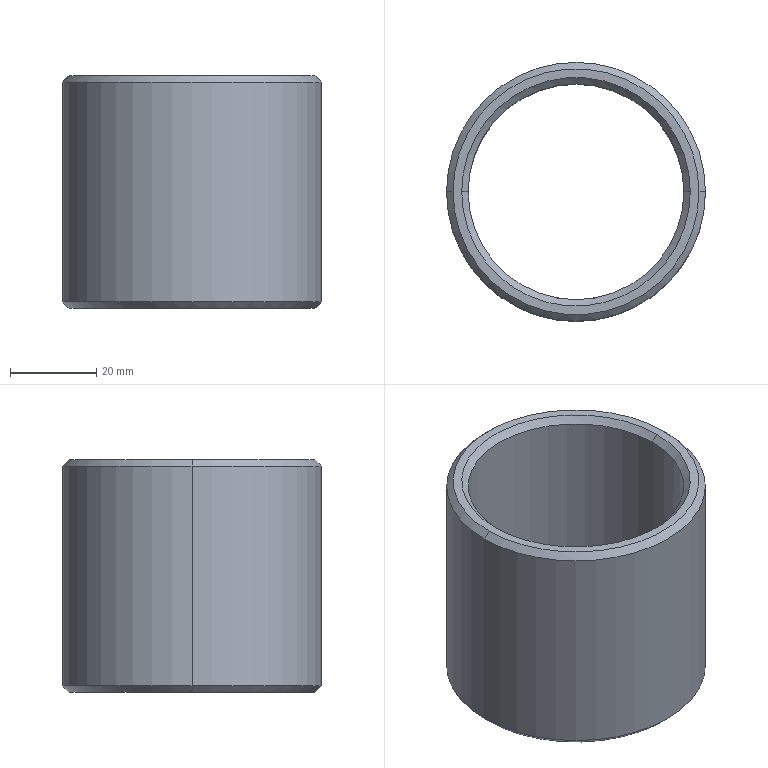Part | SolidWorks | features Chamfer 1, Extrusion 1, ICE 1, RevCut 1 | 1 solid | 18 faces | box 60 x 60 x 54 mm | volume 45325 mm3 | cone 9 | cylinder 5 | sphere 2 | plane 2 | commonest cylinder face diameters 50 x2 60 x2 6 x1
STEP:
#1=CARTESIAN_POINT('',(-25.,0.,25.5));
#2=VERTEX_POINT('',#1);
#3=CARTESIAN_POINT('',(25.,0.,25.5));
#4=VERTEX_POINT('',#3);
#5=CARTESIAN_POINT('',(0.,0.,25.5));
#6=DIRECTION('',(0.,0.,1.));
#7=DIRECTION('',(1.,0.,0.));
#8=AXIS2_PLACEMENT_3D('',#5,#6,#7);
#9=CIRCLE('',#8,25.);
#10=EDGE_CURVE('',#2,#4,#9,.T.);
#11=ORIENTED_EDGE('',*,*,#10,.F.);
#12=CARTESIAN_POINT('',(-26.5,0.,27.));
#13=VERTEX_POINT('',#12);
#14=CARTESIAN_POINT('',(-25.,0.,25.5));
#15=DIRECTION('',(-0.7071,0.,0.7071));
#16=VECTOR('',#15,1000.);
#17=LINE('',#14,#16);
#18=EDGE_CURVE('',#2,#13,#17,.T.);
#19=ORIENTED_EDGE('',*,*,#18,.T.);
#20=CARTESIAN_POINT('',(26.5,0.,27.));
#21=VERTEX_POINT('',#20);
#22=CARTESIAN_POINT('',(0.,0.,27.));
#23=DIRECTION('',(0.,0.,-1.));
#24=DIRECTION('',(1.,0.,0.));
#25=AXIS2_PLACEMENT_3D('',#22,#23,#24);
#26=CIRCLE('',#25,26.5);
#27=EDGE_CURVE('',#21,#13,#26,.T.);
#28=ORIENTED_EDGE('',*,*,#27,.F.);
#29=CARTESIAN_POINT('',(25.,0.,25.5));
#30=DIRECTION('',(0.7071,0.,0.7071));
#31=VECTOR('',#30,1000.);
#32=LINE('',#29,#31);
#33=EDGE_CURVE('',#4,#21,#32,.T.);
#34=ORIENTED_EDGE('',*,*,#33,.F.);
#35=EDGE_LOOP('',(#11,#19,#28,#34));
#36=FACE_OUTER_BOUND('',#35,.T.);
#37=CARTESIAN_POINT('',(0.,0.,25.5));
#38=DIRECTION('',(0.,0.,1.));
#39=DIRECTION('',(1.,0.,0.));
#40=AXIS2_PLACEMENT_3D('',#37,#38,#39);
#41=CONICAL_SURFACE('',#40,25.,0.7854);
#42=ADVANCED_FACE('',(#36),#41,.F.);
#43=CARTESIAN_POINT('',(28.5,0.,27.));
#44=VERTEX_POINT('',#43);
#45=CARTESIAN_POINT('',(-28.5,0.,27.));
#46=VERTEX_POINT('',#45);
#47=CARTESIAN_POINT('',(0.,0.,27.));
#48=DIRECTION('',(0.,0.,1.));
#49=DIRECTION('',(1.,0.,0.));
#50=AXIS2_PLACEMENT_3D('',#47,#48,#49);
#51=CIRCLE('',#50,28.5);
#52=EDGE_CURVE('',#44,#46,#51,.T.);
#53=ORIENTED_EDGE('',*,*,#52,.F.);
#54=CARTESIAN_POINT('',(30.,0.,25.5));
#55=VERTEX_POINT('',#54);
#56=CARTESIAN_POINT('',(28.5,0.,27.));
#57=DIRECTION('',(0.7071,0.,-0.7071));
#58=VECTOR('',#57,1000.);
#59=LINE('',#56,#58);
#60=EDGE_CURVE('',#44,#55,#59,.T.);
#61=ORIENTED_EDGE('',*,*,#60,.T.);
#62=CARTESIAN_POINT('',(-30.,0.,25.5));
#63=VERTEX_POINT('',#62);
#64=CARTESIAN_POINT('',(0.,0.,25.5));
#65=DIRECTION('',(0.,0.,-1.));
#66=DIRECTION('',(1.,0.,0.));
#67=AXIS2_PLACEMENT_3D('',#64,#65,#66);
#68=CIRCLE('',#67,30.);
#69=EDGE_CURVE('',#63,#55,#68,.T.);
#70=ORIENTED_EDGE('',*,*,#69,.F.);
#71=CARTESIAN_POINT('',(-28.5,0.,27.));
#72=DIRECTION('',(-0.7071,0.,-0.7071));
#73=VECTOR('',#72,1000.);
#74=LINE('',#71,#73);
#75=EDGE_CURVE('',#46,#63,#74,.T.);
#76=ORIENTED_EDGE('',*,*,#75,.F.);
#77=EDGE_LOOP('',(#53,#61,#70,#76));
#78=FACE_OUTER_BOUND('',#77,.T.);
#79=CARTESIAN_POINT('',(0.,0.,27.));
#80=DIRECTION('',(0.,0.,-1.));
#81=DIRECTION('',(-1.,0.,0.));
#82=AXIS2_PLACEMENT_3D('',#79,#80,#81);
#83=CONICAL_SURFACE('',#82,28.5,0.7854);
#84=ADVANCED_FACE('',(#78),#83,.T.);
#85=CARTESIAN_POINT('',(-28.5,0.,-27.));
#86=VERTEX_POINT('',#85);
#87=CARTESIAN_POINT('',(28.5,0.,-27.));
#88=VERTEX_POINT('',#87);
#89=CARTESIAN_POINT('',(0.,0.,-27.));
#90=DIRECTION('',(0.,0.,-1.));
#91=DIRECTION('',(1.,0.,0.));
#92=AXIS2_PLACEMENT_3D('',#89,#90,#91);
#93=CIRCLE('',#92,28.5);
#94=EDGE_CURVE('',#86,#88,#93,.T.);
#95=ORIENTED_EDGE('',*,*,#94,.F.);
#96=CARTESIAN_POINT('',(-30.,0.,-25.5));
#97=VERTEX_POINT('',#96);
#98=CARTESIAN_POINT('',(-30.,0.,-25.5));
#99=DIRECTION('',(-0.7071,0.,0.7071));
#100=VECTOR('',#99,1000.);
#101=LINE('',#98,#100);
#102=EDGE_CURVE('',#86,#97,#101,.T.);
#103=ORIENTED_EDGE('',*,*,#102,.T.);
#104=CARTESIAN_POINT('',(30.,0.,-25.5));
#105=VERTEX_POINT('',#104);
#106=CARTESIAN_POINT('',(0.,0.,-25.5));
#107=DIRECTION('',(0.,0.,1.));
#108=DIRECTION('',(1.,0.,0.));
#109=AXIS2_PLACEMENT_3D('',#106,#107,#108);
#110=CIRCLE('',#109,30.);
#111=EDGE_CURVE('',#105,#97,#110,.T.);
#112=ORIENTED_EDGE('',*,*,#111,.F.);
#113=CARTESIAN_POINT('',(30.,0.,-25.5));
#114=DIRECTION('',(0.7071,0.,0.7071));
#115=VECTOR('',#114,1000.);
#116=LINE('',#113,#115);
#117=EDGE_CURVE('',#88,#105,#116,.T.);
#118=ORIENTED_EDGE('',*,*,#117,.F.);
#119=EDGE_LOOP('',(#95,#103,#112,#118));
#120=FACE_OUTER_BOUND('',#119,.T.);
#121=CARTESIAN_POINT('',(0.,0.,-25.5));
#122=DIRECTION('',(0.,0.,1.));
#123=DIRECTION('',(1.,0.,0.));
#124=AXIS2_PLACEMENT_3D('',#121,#122,#123);
#125=CONICAL_SURFACE('',#124,30.,0.7854);
#126=ADVANCED_FACE('',(#120),#125,.T.);
#127=CARTESIAN_POINT('',(25.,0.,-25.5));
#128=VERTEX_POINT('',#127);
#129=CARTESIAN_POINT('',(2.983,-24.821,-25.5));
#130=VERTEX_POINT('',#129);
#131=CARTESIAN_POINT('',(0.,0.,-25.5));
#132=DIRECTION('',(0.,0.,-1.));
#133=DIRECTION('',(1.,0.,0.));
#134=AXIS2_PLACEMENT_3D('',#131,#132,#133);
#135=CIRCLE('',#134,25.);
#136=EDGE_CURVE('',#128,#130,#135,.T.);
#137=ORIENTED_EDGE('',*,*,#136,.F.);
#138=CARTESIAN_POINT('',(26.5,0.,-27.));
#139=VERTEX_POINT('',#138);
#140=CARTESIAN_POINT('',(26.5,0.,-27.));
#141=DIRECTION('',(0.7071,0.,-0.7071));
#142=VECTOR('',#141,1000.);
#143=LINE('',#140,#142);
#144=EDGE_CURVE('',#128,#139,#143,.T.);
#145=ORIENTED_EDGE('',*,*,#144,.T.);
#146=CARTESIAN_POINT('',(2.323,-26.398,-27.));
#147=VERTEX_POINT('',#146);
#148=CARTESIAN_POINT('',(0.,0.,-27.));
#149=DIRECTION('',(0.,0.,1.));
#150=DIRECTION('',(1.,0.,0.));
#151=AXIS2_PLACEMENT_3D('',#148,#149,#150);
#152=CIRCLE('',#151,26.5);
#153=EDGE_CURVE('',#147,#139,#152,.T.);
#154=ORIENTED_EDGE('',*,*,#153,.F.);
#155=CARTESIAN_POINT('',(2.323,-26.398,-27.));
#156=CARTESIAN_POINT('',(2.522,-26.155,-26.776));
#157=CARTESIAN_POINT('',(2.669,-25.899,-26.536));
#158=CARTESIAN_POINT('',(2.885,-25.37,-26.033));
#159=CARTESIAN_POINT('',(2.953,-25.095,-25.768));
#160=CARTESIAN_POINT('',(2.983,-24.821,-25.5));
#161=B_SPLINE_CURVE_WITH_KNOTS('',3,(#155,#156,#157,#158,#159,#160),.UNSPECIFIED.,.F.,.F.,(4,2,4),(0.000000339,0.00114,0.00228),.UNSPECIFIED.);
#162=EDGE_CURVE('',#147,#130,#161,.T.);
#163=ORIENTED_EDGE('',*,*,#162,.T.);
#164=EDGE_LOOP('',(#137,#145,#154,#163));
#165=FACE_OUTER_BOUND('',#164,.T.);
#166=CARTESIAN_POINT('',(0.,0.,-27.));
#167=DIRECTION('',(0.,0.,-1.));
#168=DIRECTION('',(-1.,0.,0.));
#169=AXIS2_PLACEMENT_3D('',#166,#167,#168);
#170=CONICAL_SURFACE('',#169,26.5,0.7854);
#171=ADVANCED_FACE('',(#165),#170,.F.);
#172=ORIENTED_EDGE('',*,*,#144,.F.);
#173=CARTESIAN_POINT('',(-25.,0.,-25.5));
#174=VERTEX_POINT('',#173);
#175=CARTESIAN_POINT('',(0.,0.,-25.5));
#176=DIRECTION('',(0.,0.,-1.));
#177=DIRECTION('',(1.,0.,0.));
#178=AXIS2_PLACEMENT_3D('',#175,#176,#177);
#179=CIRCLE('',#178,25.);
#180=EDGE_CURVE('',#174,#128,#179,.T.);
#181=ORIENTED_EDGE('',*,*,#180,.F.);
#182=CARTESIAN_POINT('',(-26.5,0.,-27.));
#183=VERTEX_POINT('',#182);
#184=CARTESIAN_POINT('',(-26.5,0.,-27.));
#185=DIRECTION('',(-0.7071,0.,-0.7071));
#186=VECTOR('',#185,1000.);
#187=LINE('',#184,#186);
#188=EDGE_CURVE('',#174,#183,#187,.T.);
#189=ORIENTED_EDGE('',*,*,#188,.T.);
#190=CARTESIAN_POINT('',(0.,0.,-27.));
#191=DIRECTION('',(0.,0.,1.));
#192=DIRECTION('',(1.,0.,0.));
#193=AXIS2_PLACEMENT_3D('',#190,#191,#192);
#194=CIRCLE('',#193,26.5);
#195=EDGE_CURVE('',#139,#183,#194,.T.);
#196=ORIENTED_EDGE('',*,*,#195,.F.);
#197=EDGE_LOOP('',(#172,#181,#189,#196));
#198=FACE_OUTER_BOUND('',#197,.T.);
#199=CARTESIAN_POINT('',(0.,0.,-27.));
#200=DIRECTION('',(0.,0.,-1.));
#201=DIRECTION('',(-1.,0.,0.));
#202=AXIS2_PLACEMENT_3D('',#199,#200,#201);
#203=CONICAL_SURFACE('',#202,26.5,0.7854);
#204=ADVANCED_FACE('',(#198),#203,.F.);
#205=ORIENTED_EDGE('',*,*,#10,.T.);
#206=CARTESIAN_POINT('',(25.,0.,27.));
#207=DIRECTION('',(0.,0.,-1.));
#208=VECTOR('',#207,1000.);
#209=LINE('',#206,#208);
#210=EDGE_CURVE('',#4,#128,#209,.T.);
#211=ORIENTED_EDGE('',*,*,#210,.T.);
#212=ORIENTED_EDGE('',*,*,#136,.T.);
#213=CARTESIAN_POINT('',(2.983,-24.821,19.5));
#214=VERTEX_POINT('',#213);
#215=CARTESIAN_POINT('',(2.983,-24.821,0.));
#216=DIRECTION('',(0.,0.,1.));
#217=VECTOR('',#216,1000.);
#218=LINE('',#215,#217);
#219=EDGE_CURVE('',#130,#214,#218,.T.);
#220=ORIENTED_EDGE('',*,*,#219,.T.);
#221=CARTESIAN_POINT('',(0.,-25.,22.458));
#222=VERTEX_POINT('',#221);
#223=CARTESIAN_POINT('',(0.,-25.,22.458));
#224=CARTESIAN_POINT('',(0.1961,-25.,22.458));
#225=CARTESIAN_POINT('',(0.3891,-24.998,22.439));
#226=CARTESIAN_POINT('',(0.7692,-24.989,22.365));
#227=CARTESIAN_POINT('',(0.9582,-24.982,22.308));
#228=CARTESIAN_POINT('',(1.318,-24.966,22.161));
#229=CARTESIAN_POINT('',(1.489,-24.956,22.071));
#230=CARTESIAN_POINT('',(1.814,-24.935,21.858));
#231=CARTESIAN_POINT('',(1.967,-24.923,21.734));
#232=CARTESIAN_POINT('',(2.243,-24.9,21.462));
#233=CARTESIAN_POINT('',(2.366,-24.888,21.313));
#234=CARTESIAN_POINT('',(2.585,-24.866,20.99));
#235=CARTESIAN_POINT('',(2.678,-24.856,20.818));
#236=CARTESIAN_POINT('',(2.828,-24.84,20.461));
#237=CARTESIAN_POINT('',(2.886,-24.833,20.274));
#238=CARTESIAN_POINT('',(2.963,-24.824,19.891));
#239=CARTESIAN_POINT('',(2.983,-24.821,19.696));
#240=CARTESIAN_POINT('',(2.983,-24.821,19.5));
#241=B_SPLINE_CURVE_WITH_KNOTS('',3,(#223,#224,#225,#226,#227,#228,#229,#230,#231,#232,#233,#234,#235,#236,#237,#238,#239,#240),.UNSPECIFIED.,.F.,.F.,(4,2,2,2,2,2,2,2,4),(0.01395,0.01453,0.01511,0.01569,0.01627,0.01685,0.01743,0.01801,0.01859),.UNSPECIFIED.);
#242=EDGE_CURVE('',#222,#214,#241,.T.);
#243=ORIENTED_EDGE('',*,*,#242,.F.);
#244=CARTESIAN_POINT('',(-2.983,-24.821,19.5));
#245=VERTEX_POINT('',#244);
#246=CARTESIAN_POINT('',(-2.983,-24.821,19.5));
#247=CARTESIAN_POINT('',(-2.983,-24.821,19.694));
#248=CARTESIAN_POINT('',(-2.964,-24.824,19.887));
#249=CARTESIAN_POINT('',(-2.887,-24.833,20.271));
#250=CARTESIAN_POINT('',(-2.829,-24.84,20.458));
#251=CARTESIAN_POINT('',(-2.68,-24.856,20.815));
#252=CARTESIAN_POINT('',(-2.587,-24.866,20.988));
#253=CARTESIAN_POINT('',(-2.368,-24.888,21.311));
#254=CARTESIAN_POINT('',(-2.244,-24.899,21.46));
#255=CARTESIAN_POINT('',(-1.969,-24.923,21.732));
#256=CARTESIAN_POINT('',(-1.815,-24.935,21.857));
#257=CARTESIAN_POINT('',(-1.491,-24.956,22.07));
#258=CARTESIAN_POINT('',(-1.32,-24.966,22.161));
#259=CARTESIAN_POINT('',(-0.9588,-24.982,22.308));
#260=CARTESIAN_POINT('',(-0.7702,-24.989,22.364));
#261=CARTESIAN_POINT('',(-0.3901,-24.998,22.439));
#262=CARTESIAN_POINT('',(-0.1962,-25.,22.458));
#263=CARTESIAN_POINT('',(0.,-25.,22.458));
#264=B_SPLINE_CURVE_WITH_KNOTS('',3,(#246,#247,#248,#249,#250,#251,#252,#253,#254,#255,#256,#257,#258,#259,#260,#261,#262,#263),.UNSPECIFIED.,.F.,.F.,(4,2,2,2,2,2,2,2,4),(0.009298,0.009879,0.01046,0.01104,0.01162,0.0122,0.01278,0.01337,0.01395),.UNSPECIFIED.);
#265=EDGE_CURVE('',#245,#222,#264,.T.);
#266=ORIENTED_EDGE('',*,*,#265,.F.);
#267=CARTESIAN_POINT('',(-2.983,-24.821,-25.5));
#268=VERTEX_POINT('',#267);
#269=CARTESIAN_POINT('',(-2.983,-24.821,0.));
#270=DIRECTION('',(0.,0.,-1.));
#271=VECTOR('',#270,1000.);
#272=LINE('',#269,#271);
#273=EDGE_CURVE('',#245,#268,#272,.T.);
#274=ORIENTED_EDGE('',*,*,#273,.T.);
#275=CARTESIAN_POINT('',(0.,0.,-25.5));
#276=DIRECTION('',(0.,0.,-1.));
#277=DIRECTION('',(1.,0.,0.));
#278=AXIS2_PLACEMENT_3D('',#275,#276,#277);
#279=CIRCLE('',#278,25.);
#280=EDGE_CURVE('',#268,#174,#279,.T.);
#281=ORIENTED_EDGE('',*,*,#280,.T.);
#282=CARTESIAN_POINT('',(-25.,0.,27.));
#283=DIRECTION('',(0.,0.,-1.));
#284=VECTOR('',#283,1000.);
#285=LINE('',#282,#284);
#286=EDGE_CURVE('',#2,#174,#285,.T.);
#287=ORIENTED_EDGE('',*,*,#286,.F.);
#288=EDGE_LOOP('',(#205,#211,#212,#220,#243,#266,#274,#281,#287));
#289=FACE_OUTER_BOUND('',#288,.T.);
#290=CARTESIAN_POINT('',(0.,0.,27.));
#291=DIRECTION('',(0.,0.,-1.));
#292=DIRECTION('',(-1.,0.,0.));
#293=AXIS2_PLACEMENT_3D('',#290,#291,#292);
#294=CYLINDRICAL_SURFACE('',#293,25.);
#295=ADVANCED_FACE('',(#289),#294,.F.);
#296=ORIENTED_EDGE('',*,*,#69,.T.);
#297=CARTESIAN_POINT('',(30.,0.,27.));
#298=DIRECTION('',(0.,0.,-1.));
#299=VECTOR('',#298,1000.);
#300=LINE('',#297,#299);
#301=EDGE_CURVE('',#55,#105,#300,.T.);
#302=ORIENTED_EDGE('',*,*,#301,.T.);
#303=ORIENTED_EDGE('',*,*,#111,.T.);
#304=CARTESIAN_POINT('',(-30.,0.,27.));
#305=DIRECTION('',(0.,0.,-1.));
#306=VECTOR('',#305,1000.);
#307=LINE('',#304,#306);
#308=EDGE_CURVE('',#63,#97,#307,.T.);
#309=ORIENTED_EDGE('',*,*,#308,.F.);
#310=EDGE_LOOP('',(#296,#302,#303,#309));
#311=FACE_OUTER_BOUND('',#310,.T.);
#312=CARTESIAN_POINT('',(0.,0.,27.));
#313=DIRECTION('',(0.,0.,-1.));
#314=DIRECTION('',(-1.,0.,0.));
#315=AXIS2_PLACEMENT_3D('',#312,#313,#314);
#316=CYLINDRICAL_SURFACE('',#315,30.);
#317=ADVANCED_FACE('',(#311),#316,.T.);
#318=CARTESIAN_POINT('',(0.,-27.5,19.5));
#319=VERTEX_POINT('',#318);
#320=CARTESIAN_POINT('',(0.,-24.5,19.5));
#321=DIRECTION('',(0.,0.,-1.));
#322=DIRECTION('',(-1.,0.,0.));
#323=AXIS2_PLACEMENT_3D('',#320,#321,#322);
#324=CIRCLE('',#323,3.);
#325=EDGE_CURVE('',#214,#319,#324,.T.);
#326=ORIENTED_EDGE('',*,*,#325,.T.);
#327=CARTESIAN_POINT('',(0.,-24.5,19.5));
#328=DIRECTION('',(-1.,0.,0.));
#329=DIRECTION('',(0.,0.,1.));
#330=AXIS2_PLACEMENT_3D('',#327,#328,#329);
#331=CIRCLE('',#330,3.);
#332=EDGE_CURVE('',#319,#222,#331,.T.);
#333=ORIENTED_EDGE('',*,*,#332,.T.);
#334=ORIENTED_EDGE('',*,*,#242,.T.);
#335=EDGE_LOOP('',(#326,#333,#334));
#336=FACE_OUTER_BOUND('',#335,.T.);
#337=CARTESIAN_POINT('',(0.,-24.5,19.5));
#338=DIRECTION('',(1.,0.,0.));
#339=DIRECTION('',(0.,0.,1.));
#340=AXIS2_PLACEMENT_3D('',#337,#338,#339);
#341=SPHERICAL_SURFACE('',#340,3.);
#342=ADVANCED_FACE('',(#336),#341,.F.);
#343=ORIENTED_EDGE('',*,*,#332,.F.);
#344=CARTESIAN_POINT('',(0.,-24.5,19.5));
#345=DIRECTION('',(0.,0.,-1.));
#346=DIRECTION('',(-1.,0.,0.));
#347=AXIS2_PLACEMENT_3D('',#344,#345,#346);
#348=CIRCLE('',#347,3.);
#349=EDGE_CURVE('',#319,#245,#348,.T.);
#350=ORIENTED_EDGE('',*,*,#349,.T.);
#351=ORIENTED_EDGE('',*,*,#265,.T.);
#352=EDGE_LOOP('',(#343,#350,#351));
#353=FACE_OUTER_BOUND('',#352,.T.);
#354=CARTESIAN_POINT('',(0.,-24.5,19.5));
#355=DIRECTION('',(1.,0.,0.));
#356=DIRECTION('',(0.,0.,1.));
#357=AXIS2_PLACEMENT_3D('',#354,#355,#356);
#358=SPHERICAL_SURFACE('',#357,3.);
#359=ADVANCED_FACE('',(#353),#358,.F.);
#360=CARTESIAN_POINT('',(0.,0.,27.));
#361=DIRECTION('',(0.,0.,1.));
#362=DIRECTION('',(1.,0.,0.));
#363=AXIS2_PLACEMENT_3D('',#360,#361,#362);
#364=CIRCLE('',#363,28.5);
#365=EDGE_CURVE('',#46,#44,#364,.T.);
#366=ORIENTED_EDGE('',*,*,#365,.T.);
#367=ORIENTED_EDGE('',*,*,#52,.T.);
#368=EDGE_LOOP('',(#366,#367));
#369=FACE_OUTER_BOUND('',#368,.T.);
#370=ORIENTED_EDGE('',*,*,#27,.T.);
#371=CARTESIAN_POINT('',(0.,0.,27.));
#372=DIRECTION('',(0.,0.,-1.));
#373=DIRECTION('',(1.,0.,0.));
#374=AXIS2_PLACEMENT_3D('',#371,#372,#373);
#375=CIRCLE('',#374,26.5);
#376=EDGE_CURVE('',#13,#21,#375,.T.);
#377=ORIENTED_EDGE('',*,*,#376,.T.);
#378=EDGE_LOOP('',(#370,#377));
#379=FACE_BOUND('',#378,.T.);
#380=CARTESIAN_POINT('',(0.,0.,27.));
#381=DIRECTION('',(0.,0.,1.));
#382=DIRECTION('',(1.,0.,0.));
#383=AXIS2_PLACEMENT_3D('',#380,#381,#382);
#384=PLANE('',#383);
#385=ADVANCED_FACE('',(#369,#379),#384,.T.);
#386=ORIENTED_EDGE('',*,*,#153,.T.);
#387=ORIENTED_EDGE('',*,*,#195,.T.);
#388=CARTESIAN_POINT('',(-2.323,-26.398,-27.));
#389=VERTEX_POINT('',#388);
#390=CARTESIAN_POINT('',(0.,0.,-27.));
#391=DIRECTION('',(0.,0.,1.));
#392=DIRECTION('',(1.,0.,0.));
#393=AXIS2_PLACEMENT_3D('',#390,#391,#392);
#394=CIRCLE('',#393,26.5);
#395=EDGE_CURVE('',#183,#389,#394,.T.);
#396=ORIENTED_EDGE('',*,*,#395,.T.);
#397=CARTESIAN_POINT('',(0.,-24.5,-27.));
#398=DIRECTION('',(0.,0.,-1.));
#399=DIRECTION('',(-1.,0.,0.));
#400=AXIS2_PLACEMENT_3D('',#397,#398,#399);
#401=CIRCLE('',#400,3.);
#402=EDGE_CURVE('',#147,#389,#401,.T.);
#403=ORIENTED_EDGE('',*,*,#402,.F.);
#404=EDGE_LOOP('',(#386,#387,#396,#403));
#405=FACE_BOUND('',#404,.T.);
#406=CARTESIAN_POINT('',(0.,0.,-27.));
#407=DIRECTION('',(0.,0.,-1.));
#408=DIRECTION('',(1.,0.,0.));
#409=AXIS2_PLACEMENT_3D('',#406,#407,#408);
#410=CIRCLE('',#409,28.5);
#411=EDGE_CURVE('',#88,#86,#410,.T.);
#412=ORIENTED_EDGE('',*,*,#411,.T.);
#413=ORIENTED_EDGE('',*,*,#94,.T.);
#414=EDGE_LOOP('',(#412,#413));
#415=FACE_OUTER_BOUND('',#414,.T.);
#416=CARTESIAN_POINT('',(0.,0.,-27.));
#417=DIRECTION('',(0.,0.,1.));
#418=DIRECTION('',(1.,0.,0.));
#419=AXIS2_PLACEMENT_3D('',#416,#417,#418);
#420=PLANE('',#419);
#421=ADVANCED_FACE('',(#405,#415),#420,.F.);
#422=ORIENTED_EDGE('',*,*,#301,.F.);
#423=CARTESIAN_POINT('',(0.,0.,25.5));
#424=DIRECTION('',(0.,0.,-1.));
#425=DIRECTION('',(1.,0.,0.));
#426=AXIS2_PLACEMENT_3D('',#423,#424,#425);
#427=CIRCLE('',#426,30.);
#428=EDGE_CURVE('',#55,#63,#427,.T.);
#429=ORIENTED_EDGE('',*,*,#428,.T.);
#430=ORIENTED_EDGE('',*,*,#308,.T.);
#431=CARTESIAN_POINT('',(0.,0.,-25.5));
#432=DIRECTION('',(0.,0.,1.));
#433=DIRECTION('',(1.,0.,0.));
#434=AXIS2_PLACEMENT_3D('',#431,#432,#433);
#435=CIRCLE('',#434,30.);
#436=EDGE_CURVE('',#97,#105,#435,.T.);
#437=ORIENTED_EDGE('',*,*,#436,.T.);
#438=EDGE_LOOP('',(#422,#429,#430,#437));
#439=FACE_OUTER_BOUND('',#438,.T.);
#440=CARTESIAN_POINT('',(0.,0.,27.));
#441=DIRECTION('',(0.,0.,-1.));
#442=DIRECTION('',(-1.,0.,0.));
#443=AXIS2_PLACEMENT_3D('',#440,#441,#442);
#444=CYLINDRICAL_SURFACE('',#443,30.);
#445=ADVANCED_FACE('',(#439),#444,.T.);
#446=ORIENTED_EDGE('',*,*,#210,.F.);
#447=CARTESIAN_POINT('',(0.,0.,25.5));
#448=DIRECTION('',(0.,0.,1.));
#449=DIRECTION('',(1.,0.,0.));
#450=AXIS2_PLACEMENT_3D('',#447,#448,#449);
#451=CIRCLE('',#450,25.);
#452=EDGE_CURVE('',#4,#2,#451,.T.);
#453=ORIENTED_EDGE('',*,*,#452,.T.);
#454=ORIENTED_EDGE('',*,*,#286,.T.);
#455=ORIENTED_EDGE('',*,*,#180,.T.);
#456=EDGE_LOOP('',(#446,#453,#454,#455));
#457=FACE_OUTER_BOUND('',#456,.T.);
#458=CARTESIAN_POINT('',(0.,0.,27.));
#459=DIRECTION('',(0.,0.,-1.));
#460=DIRECTION('',(-1.,0.,0.));
#461=AXIS2_PLACEMENT_3D('',#458,#459,#460);
#462=CYLINDRICAL_SURFACE('',#461,25.);
#463=ADVANCED_FACE('',(#457),#462,.F.);
#464=ORIENTED_EDGE('',*,*,#188,.F.);
#465=ORIENTED_EDGE('',*,*,#280,.F.);
#466=CARTESIAN_POINT('',(-2.983,-24.821,-25.5));
#467=CARTESIAN_POINT('',(-2.953,-25.095,-25.768));
#468=CARTESIAN_POINT('',(-2.887,-25.365,-26.028));
#469=CARTESIAN_POINT('',(-2.671,-25.895,-26.532));
#470=CARTESIAN_POINT('',(-2.521,-26.156,-26.776));
#471=CARTESIAN_POINT('',(-2.323,-26.398,-27.));
#472=B_SPLINE_CURVE_WITH_KNOTS('',3,(#466,#467,#468,#469,#470,#471),.UNSPECIFIED.,.F.,.F.,(4,2,4),(0.000000284,0.001141,0.002283),.UNSPECIFIED.);
#473=EDGE_CURVE('',#268,#389,#472,.T.);
#474=ORIENTED_EDGE('',*,*,#473,.T.);
#475=ORIENTED_EDGE('',*,*,#395,.F.);
#476=EDGE_LOOP('',(#464,#465,#474,#475));
#477=FACE_OUTER_BOUND('',#476,.T.);
#478=CARTESIAN_POINT('',(0.,0.,-27.));
#479=DIRECTION('',(0.,0.,-1.));
#480=DIRECTION('',(-1.,0.,0.));
#481=AXIS2_PLACEMENT_3D('',#478,#479,#480);
#482=CONICAL_SURFACE('',#481,26.5,0.7854);
#483=ADVANCED_FACE('',(#477),#482,.F.);
#484=ORIENTED_EDGE('',*,*,#102,.F.);
#485=ORIENTED_EDGE('',*,*,#411,.F.);
#486=ORIENTED_EDGE('',*,*,#117,.T.);
#487=ORIENTED_EDGE('',*,*,#436,.F.);
#488=EDGE_LOOP('',(#484,#485,#486,#487));
#489=FACE_OUTER_BOUND('',#488,.T.);
#490=CARTESIAN_POINT('',(0.,0.,-25.5));
#491=DIRECTION('',(0.,0.,1.));
#492=DIRECTION('',(1.,0.,0.));
#493=AXIS2_PLACEMENT_3D('',#490,#491,#492);
#494=CONICAL_SURFACE('',#493,30.,0.7854);
#495=ADVANCED_FACE('',(#489),#494,.T.);
#496=ORIENTED_EDGE('',*,*,#60,.F.);
#497=ORIENTED_EDGE('',*,*,#365,.F.);
#498=ORIENTED_EDGE('',*,*,#75,.T.);
#499=ORIENTED_EDGE('',*,*,#428,.F.);
#500=EDGE_LOOP('',(#496,#497,#498,#499));
#501=FACE_OUTER_BOUND('',#500,.T.);
#502=CARTESIAN_POINT('',(0.,0.,27.));
#503=DIRECTION('',(0.,0.,-1.));
#504=DIRECTION('',(-1.,0.,0.));
#505=AXIS2_PLACEMENT_3D('',#502,#503,#504);
#506=CONICAL_SURFACE('',#505,28.5,0.7854);
#507=ADVANCED_FACE('',(#501),#506,.T.);
#508=ORIENTED_EDGE('',*,*,#18,.F.);
#509=ORIENTED_EDGE('',*,*,#452,.F.);
#510=ORIENTED_EDGE('',*,*,#33,.T.);
#511=ORIENTED_EDGE('',*,*,#376,.F.);
#512=EDGE_LOOP('',(#508,#509,#510,#511));
#513=FACE_OUTER_BOUND('',#512,.T.);
#514=CARTESIAN_POINT('',(0.,0.,25.5));
#515=DIRECTION('',(0.,0.,1.));
#516=DIRECTION('',(1.,0.,0.));
#517=AXIS2_PLACEMENT_3D('',#514,#515,#516);
#518=CONICAL_SURFACE('',#517,25.,0.7854);
#519=ADVANCED_FACE('',(#513),#518,.F.);
#520=ORIENTED_EDGE('',*,*,#162,.F.);
#521=ORIENTED_EDGE('',*,*,#402,.T.);
#522=ORIENTED_EDGE('',*,*,#473,.F.);
#523=ORIENTED_EDGE('',*,*,#273,.F.);
#524=ORIENTED_EDGE('',*,*,#349,.F.);
#525=ORIENTED_EDGE('',*,*,#325,.F.);
#526=ORIENTED_EDGE('',*,*,#219,.F.);
#527=EDGE_LOOP('',(#520,#521,#522,#523,#524,#525,#526));
#528=FACE_OUTER_BOUND('',#527,.T.);
#529=CARTESIAN_POINT('',(0.,-24.5,27.001));
#530=DIRECTION('',(0.,0.,-1.));
#531=DIRECTION('',(-1.,0.,0.));
#532=AXIS2_PLACEMENT_3D('',#529,#530,#531);
#533=CYLINDRICAL_SURFACE('',#532,3.);
#534=ADVANCED_FACE('',(#528),#533,.F.);
#535=CLOSED_SHELL('',(#42,#84,#126,#171,#204,#295,#317,#342,#359,#385,#421,#445,#463,#483,#495,#507,#519,#534));
#536=MANIFOLD_SOLID_BREP('',#535);
#537=CARTESIAN_POINT('',(0.,0.,0.));
#538=DIRECTION('',(0.,0.,1.));
#539=DIRECTION('',(1.,0.,0.));
#540=AXIS2_PLACEMENT_3D('',#537,#538,#539);
#541=(LENGTH_UNIT()NAMED_UNIT(*)SI_UNIT(.MILLI.,.METRE.));
#542=UNCERTAINTY_MEASURE_WITH_UNIT(LENGTH_MEASURE(0.00001),#541,'','');
#543=(NAMED_UNIT(*)PLANE_ANGLE_UNIT()SI_UNIT($,.RADIAN.));
#544=(NAMED_UNIT(*)SI_UNIT($,.STERADIAN.)SOLID_ANGLE_UNIT());
#545=(GEOMETRIC_REPRESENTATION_CONTEXT(3)GLOBAL_UNCERTAINTY_ASSIGNED_CONTEXT((#542))GLOBAL_UNIT_ASSIGNED_CONTEXT((#541,#543,#544))REPRESENTATION_CONTEXT('',''));
#546=ADVANCED_BREP_SHAPE_REPRESENTATION('',(#536,#540),#545);